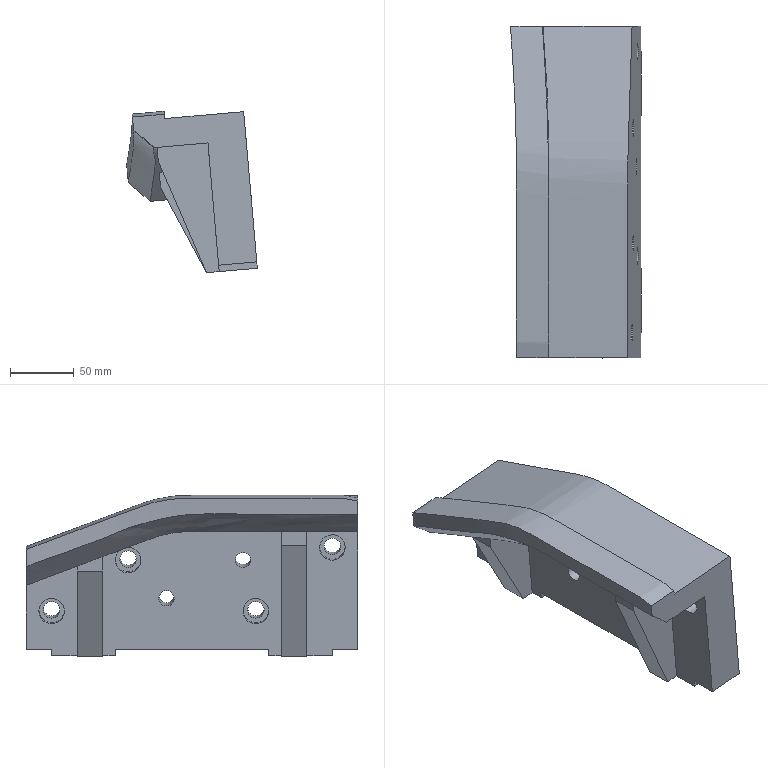Part | NX | features solid 2 | 1 solid | 43 faces | box 102.383 x 260 x 126.445 mm | volume 1293464 mm3 | plane 27 | cylinder 10 | spline 6 | commonest cylinder face diameters 13 x4 20 x4 12 x2